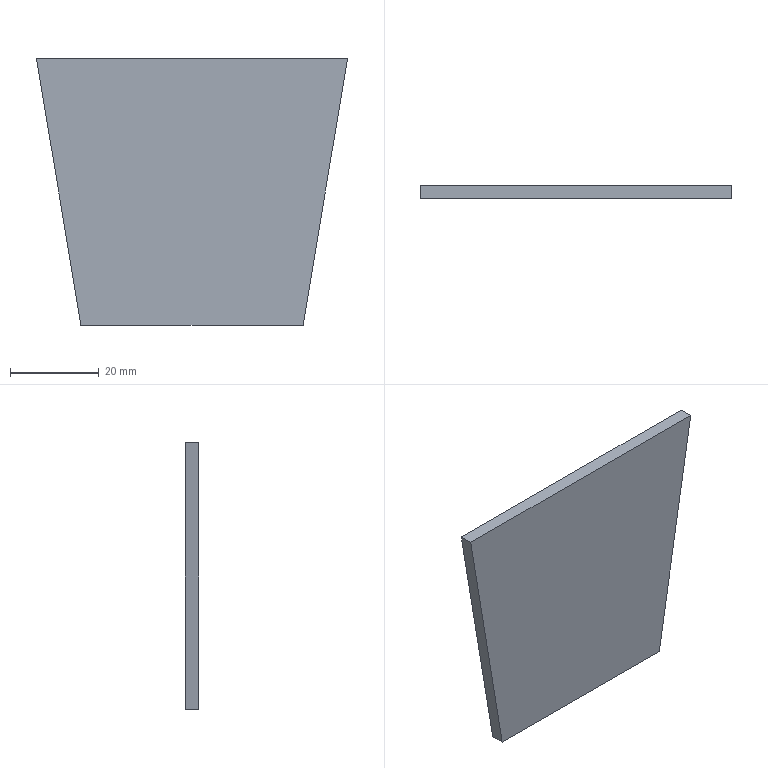Part | SolidWorks | features Extrusion 1 | 1 solid | 6 faces | box 70 x 3 x 60 mm | volume 10800 mm3 | plane 6
STEP:
#1=CARTESIAN_POINT('',(35.,0.,30.));
#2=VERTEX_POINT('',#1);
#3=CARTESIAN_POINT('',(25.,0.,-30.));
#4=VERTEX_POINT('',#3);
#5=CARTESIAN_POINT('',(25.,0.,-30.));
#6=DIRECTION('',(-0.1644,0.,-0.9864));
#7=VECTOR('',#6,1000.);
#8=LINE('',#5,#7);
#9=EDGE_CURVE('',#2,#4,#8,.T.);
#10=ORIENTED_EDGE('',*,*,#9,.T.);
#11=CARTESIAN_POINT('',(25.,3.,-30.));
#12=VERTEX_POINT('',#11);
#13=CARTESIAN_POINT('',(25.,3.,-30.));
#14=DIRECTION('',(0.,-1.,0.));
#15=VECTOR('',#14,1000.);
#16=LINE('',#13,#15);
#17=EDGE_CURVE('',#12,#4,#16,.T.);
#18=ORIENTED_EDGE('',*,*,#17,.F.);
#19=CARTESIAN_POINT('',(35.,3.,30.));
#20=VERTEX_POINT('',#19);
#21=CARTESIAN_POINT('',(25.,3.,-30.));
#22=DIRECTION('',(-0.1644,0.,-0.9864));
#23=VECTOR('',#22,1000.);
#24=LINE('',#21,#23);
#25=EDGE_CURVE('',#20,#12,#24,.T.);
#26=ORIENTED_EDGE('',*,*,#25,.F.);
#27=CARTESIAN_POINT('',(35.,3.,30.));
#28=DIRECTION('',(0.,-1.,0.));
#29=VECTOR('',#28,1000.);
#30=LINE('',#27,#29);
#31=EDGE_CURVE('',#20,#2,#30,.T.);
#32=ORIENTED_EDGE('',*,*,#31,.T.);
#33=EDGE_LOOP('',(#10,#18,#26,#32));
#34=FACE_OUTER_BOUND('',#33,.T.);
#35=CARTESIAN_POINT('',(25.,3.,-30.));
#36=DIRECTION('',(-0.9864,0.,0.1644));
#37=DIRECTION('',(0.1644,0.,0.9864));
#38=AXIS2_PLACEMENT_3D('',#35,#36,#37);
#39=PLANE('',#38);
#40=ADVANCED_FACE('',(#34),#39,.F.);
#41=CARTESIAN_POINT('',(-25.,0.,-30.));
#42=VERTEX_POINT('',#41);
#43=CARTESIAN_POINT('',(-25.,0.,-30.));
#44=DIRECTION('',(-1.,0.,0.));
#45=VECTOR('',#44,1000.);
#46=LINE('',#43,#45);
#47=EDGE_CURVE('',#4,#42,#46,.T.);
#48=ORIENTED_EDGE('',*,*,#47,.T.);
#49=CARTESIAN_POINT('',(-25.,3.,-30.));
#50=VERTEX_POINT('',#49);
#51=CARTESIAN_POINT('',(-25.,3.,-30.));
#52=DIRECTION('',(0.,-1.,0.));
#53=VECTOR('',#52,1000.);
#54=LINE('',#51,#53);
#55=EDGE_CURVE('',#50,#42,#54,.T.);
#56=ORIENTED_EDGE('',*,*,#55,.F.);
#57=CARTESIAN_POINT('',(-25.,3.,-30.));
#58=DIRECTION('',(-1.,0.,0.));
#59=VECTOR('',#58,1000.);
#60=LINE('',#57,#59);
#61=EDGE_CURVE('',#12,#50,#60,.T.);
#62=ORIENTED_EDGE('',*,*,#61,.F.);
#63=ORIENTED_EDGE('',*,*,#17,.T.);
#64=EDGE_LOOP('',(#48,#56,#62,#63));
#65=FACE_OUTER_BOUND('',#64,.T.);
#66=CARTESIAN_POINT('',(-25.,3.,-30.));
#67=DIRECTION('',(0.,0.,1.));
#68=DIRECTION('',(1.,0.,0.));
#69=AXIS2_PLACEMENT_3D('',#66,#67,#68);
#70=PLANE('',#69);
#71=ADVANCED_FACE('',(#65),#70,.F.);
#72=CARTESIAN_POINT('',(-35.,0.,30.));
#73=VERTEX_POINT('',#72);
#74=CARTESIAN_POINT('',(-25.,0.,-30.));
#75=DIRECTION('',(-0.1644,0.,0.9864));
#76=VECTOR('',#75,1000.);
#77=LINE('',#74,#76);
#78=EDGE_CURVE('',#42,#73,#77,.T.);
#79=ORIENTED_EDGE('',*,*,#78,.T.);
#80=CARTESIAN_POINT('',(-35.,3.,30.));
#81=VERTEX_POINT('',#80);
#82=CARTESIAN_POINT('',(-35.,3.,30.));
#83=DIRECTION('',(0.,-1.,0.));
#84=VECTOR('',#83,1000.);
#85=LINE('',#82,#84);
#86=EDGE_CURVE('',#81,#73,#85,.T.);
#87=ORIENTED_EDGE('',*,*,#86,.F.);
#88=CARTESIAN_POINT('',(-25.,3.,-30.));
#89=DIRECTION('',(-0.1644,0.,0.9864));
#90=VECTOR('',#89,1000.);
#91=LINE('',#88,#90);
#92=EDGE_CURVE('',#50,#81,#91,.T.);
#93=ORIENTED_EDGE('',*,*,#92,.F.);
#94=ORIENTED_EDGE('',*,*,#55,.T.);
#95=EDGE_LOOP('',(#79,#87,#93,#94));
#96=FACE_OUTER_BOUND('',#95,.T.);
#97=CARTESIAN_POINT('',(-25.,3.,-30.));
#98=DIRECTION('',(0.9864,0.,0.1644));
#99=DIRECTION('',(0.1644,0.,-0.9864));
#100=AXIS2_PLACEMENT_3D('',#97,#98,#99);
#101=PLANE('',#100);
#102=ADVANCED_FACE('',(#96),#101,.F.);
#103=CARTESIAN_POINT('',(-35.,0.,30.));
#104=DIRECTION('',(1.,0.,0.));
#105=VECTOR('',#104,1000.);
#106=LINE('',#103,#105);
#107=EDGE_CURVE('',#73,#2,#106,.T.);
#108=ORIENTED_EDGE('',*,*,#107,.T.);
#109=ORIENTED_EDGE('',*,*,#31,.F.);
#110=CARTESIAN_POINT('',(-35.,3.,30.));
#111=DIRECTION('',(1.,0.,0.));
#112=VECTOR('',#111,1000.);
#113=LINE('',#110,#112);
#114=EDGE_CURVE('',#81,#20,#113,.T.);
#115=ORIENTED_EDGE('',*,*,#114,.F.);
#116=ORIENTED_EDGE('',*,*,#86,.T.);
#117=EDGE_LOOP('',(#108,#109,#115,#116));
#118=FACE_OUTER_BOUND('',#117,.T.);
#119=CARTESIAN_POINT('',(-35.,3.,30.));
#120=DIRECTION('',(0.,0.,-1.));
#121=DIRECTION('',(-1.,0.,0.));
#122=AXIS2_PLACEMENT_3D('',#119,#120,#121);
#123=PLANE('',#122);
#124=ADVANCED_FACE('',(#118),#123,.F.);
#125=ORIENTED_EDGE('',*,*,#25,.T.);
#126=ORIENTED_EDGE('',*,*,#61,.T.);
#127=ORIENTED_EDGE('',*,*,#92,.T.);
#128=ORIENTED_EDGE('',*,*,#114,.T.);
#129=EDGE_LOOP('',(#125,#126,#127,#128));
#130=FACE_OUTER_BOUND('',#129,.T.);
#131=CARTESIAN_POINT('',(0.,3.,0.));
#132=DIRECTION('',(0.,1.,0.));
#133=DIRECTION('',(0.,0.,1.));
#134=AXIS2_PLACEMENT_3D('',#131,#132,#133);
#135=PLANE('',#134);
#136=ADVANCED_FACE('',(#130),#135,.T.);
#137=ORIENTED_EDGE('',*,*,#9,.F.);
#138=ORIENTED_EDGE('',*,*,#107,.F.);
#139=ORIENTED_EDGE('',*,*,#78,.F.);
#140=ORIENTED_EDGE('',*,*,#47,.F.);
#141=EDGE_LOOP('',(#137,#138,#139,#140));
#142=FACE_OUTER_BOUND('',#141,.T.);
#143=CARTESIAN_POINT('',(0.,0.,0.));
#144=DIRECTION('',(0.,1.,0.));
#145=DIRECTION('',(0.,0.,1.));
#146=AXIS2_PLACEMENT_3D('',#143,#144,#145);
#147=PLANE('',#146);
#148=ADVANCED_FACE('',(#142),#147,.F.);
#149=CLOSED_SHELL('',(#40,#71,#102,#124,#136,#148));
#150=MANIFOLD_SOLID_BREP('',#149);
#151=CARTESIAN_POINT('',(0.,0.,0.));
#152=DIRECTION('',(0.,0.,1.));
#153=DIRECTION('',(1.,0.,0.));
#154=AXIS2_PLACEMENT_3D('',#151,#152,#153);
#155=(LENGTH_UNIT()NAMED_UNIT(*)SI_UNIT(.MILLI.,.METRE.));
#156=UNCERTAINTY_MEASURE_WITH_UNIT(LENGTH_MEASURE(0.00001),#155,'','');
#157=(NAMED_UNIT(*)PLANE_ANGLE_UNIT()SI_UNIT($,.RADIAN.));
#158=(NAMED_UNIT(*)SI_UNIT($,.STERADIAN.)SOLID_ANGLE_UNIT());
#159=(GEOMETRIC_REPRESENTATION_CONTEXT(3)GLOBAL_UNCERTAINTY_ASSIGNED_CONTEXT((#156))GLOBAL_UNIT_ASSIGNED_CONTEXT((#155,#157,#158))REPRESENTATION_CONTEXT('',''));
#160=ADVANCED_BREP_SHAPE_REPRESENTATION('',(#150,#154),#159);